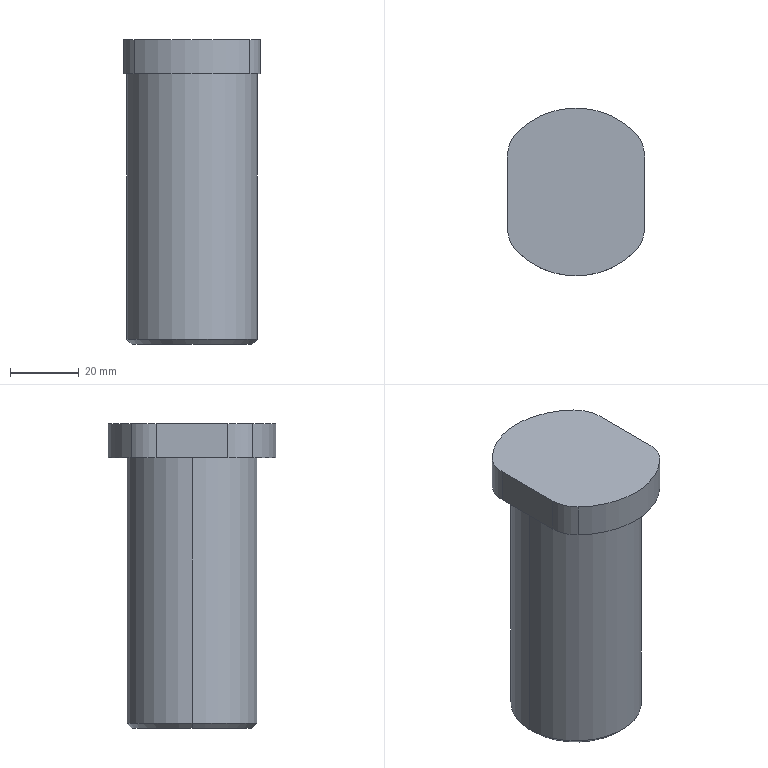Part | SolidWorks | features BaseBody 1 | 1 solid | 19 faces | box 40 x 49 x 89 mm | volume 90205 mm3 | cylinder 10 | plane 5 | cone 4 | commonest cylinder face diameters 20 x4 21 x2 38 x2 49 x2
STEP:
#1=CARTESIAN_POINT('',(-217.5,-135.,-429.5));
#2=VERTEX_POINT('',#1);
#3=CARTESIAN_POINT('',(-182.5,-135.,-429.5));
#4=VERTEX_POINT('',#3);
#5=CARTESIAN_POINT('',(-200.,-135.,-429.5));
#6=DIRECTION('',(0.,0.,-1.));
#7=DIRECTION('',(1.,0.,0.));
#8=AXIS2_PLACEMENT_3D('',#5,#6,#7);
#9=CIRCLE('',#8,17.5);
#10=EDGE_CURVE('',#2,#4,#9,.T.);
#11=ORIENTED_EDGE('',*,*,#10,.F.);
#12=CARTESIAN_POINT('',(-219.,-135.,-428.));
#13=VERTEX_POINT('',#12);
#14=CARTESIAN_POINT('',(-217.5,-135.,-429.5));
#15=DIRECTION('',(-0.7071,0.,0.7071));
#16=VECTOR('',#15,1000.);
#17=LINE('',#14,#16);
#18=EDGE_CURVE('',#2,#13,#17,.T.);
#19=ORIENTED_EDGE('',*,*,#18,.T.);
#20=CARTESIAN_POINT('',(-181.,-135.,-428.));
#21=VERTEX_POINT('',#20);
#22=CARTESIAN_POINT('',(-200.,-135.,-428.));
#23=DIRECTION('',(0.,0.,1.));
#24=DIRECTION('',(1.,0.,0.));
#25=AXIS2_PLACEMENT_3D('',#22,#23,#24);
#26=CIRCLE('',#25,19.);
#27=EDGE_CURVE('',#21,#13,#26,.T.);
#28=ORIENTED_EDGE('',*,*,#27,.F.);
#29=CARTESIAN_POINT('',(-182.5,-135.,-429.5));
#30=DIRECTION('',(0.7071,0.,0.7071));
#31=VECTOR('',#30,1000.);
#32=LINE('',#29,#31);
#33=EDGE_CURVE('',#4,#21,#32,.T.);
#34=ORIENTED_EDGE('',*,*,#33,.F.);
#35=EDGE_LOOP('',(#11,#19,#28,#34));
#36=FACE_OUTER_BOUND('',#35,.T.);
#37=CARTESIAN_POINT('',(-200.,-135.,-429.5));
#38=DIRECTION('',(0.,0.,1.));
#39=DIRECTION('',(1.,0.,0.));
#40=AXIS2_PLACEMENT_3D('',#37,#38,#39);
#41=CONICAL_SURFACE('',#40,17.5,0.7854);
#42=ADVANCED_FACE('',(#36),#41,.T.);
#43=CARTESIAN_POINT('',(-210.5,-135.,-429.5));
#44=VERTEX_POINT('',#43);
#45=CARTESIAN_POINT('',(-189.5,-135.,-429.5));
#46=VERTEX_POINT('',#45);
#47=CARTESIAN_POINT('',(-200.,-135.,-429.5));
#48=DIRECTION('',(0.,0.,1.));
#49=DIRECTION('',(1.,0.,0.));
#50=AXIS2_PLACEMENT_3D('',#47,#48,#49);
#51=CIRCLE('',#50,10.5);
#52=EDGE_CURVE('',#44,#46,#51,.T.);
#53=ORIENTED_EDGE('',*,*,#52,.F.);
#54=CARTESIAN_POINT('',(-210.5,-135.,-384.5));
#55=VERTEX_POINT('',#54);
#56=CARTESIAN_POINT('',(-210.5,-135.,-414.5));
#57=DIRECTION('',(0.,0.,1.));
#58=VECTOR('',#57,1000.);
#59=LINE('',#56,#58);
#60=EDGE_CURVE('',#44,#55,#59,.T.);
#61=ORIENTED_EDGE('',*,*,#60,.T.);
#62=CARTESIAN_POINT('',(-189.5,-135.,-384.5));
#63=VERTEX_POINT('',#62);
#64=CARTESIAN_POINT('',(-200.,-135.,-384.5));
#65=DIRECTION('',(0.,0.,1.));
#66=DIRECTION('',(1.,0.,0.));
#67=AXIS2_PLACEMENT_3D('',#64,#65,#66);
#68=CIRCLE('',#67,10.5);
#69=EDGE_CURVE('',#55,#63,#68,.T.);
#70=ORIENTED_EDGE('',*,*,#69,.T.);
#71=CARTESIAN_POINT('',(-189.5,-135.,-414.5));
#72=DIRECTION('',(0.,0.,1.));
#73=VECTOR('',#72,1000.);
#74=LINE('',#71,#73);
#75=EDGE_CURVE('',#46,#63,#74,.T.);
#76=ORIENTED_EDGE('',*,*,#75,.F.);
#77=EDGE_LOOP('',(#53,#61,#70,#76));
#78=FACE_OUTER_BOUND('',#77,.T.);
#79=CARTESIAN_POINT('',(-200.,-135.,-414.5));
#80=DIRECTION('',(0.,0.,1.));
#81=DIRECTION('',(1.,0.,0.));
#82=AXIS2_PLACEMENT_3D('',#79,#80,#81);
#83=CYLINDRICAL_SURFACE('',#82,10.5);
#84=ADVANCED_FACE('',(#78),#83,.F.);
#85=CARTESIAN_POINT('',(-200.,-135.,-378.191));
#86=VERTEX_POINT('',#85);
#87=CARTESIAN_POINT('',(-210.5,-135.,-384.5));
#88=DIRECTION('',(-0.8572,0.,-0.515));
#89=VECTOR('',#88,1000.);
#90=LINE('',#87,#89);
#91=EDGE_CURVE('',#86,#55,#90,.T.);
#92=ORIENTED_EDGE('',*,*,#91,.F.);
#93=CARTESIAN_POINT('',(-189.5,-135.,-384.5));
#94=DIRECTION('',(0.8572,0.,-0.515));
#95=VECTOR('',#94,1000.);
#96=LINE('',#93,#95);
#97=EDGE_CURVE('',#86,#63,#96,.T.);
#98=ORIENTED_EDGE('',*,*,#97,.T.);
#99=ORIENTED_EDGE('',*,*,#69,.F.);
#100=EDGE_LOOP('',(#92,#98,#99));
#101=FACE_OUTER_BOUND('',#100,.T.);
#102=CARTESIAN_POINT('',(-200.,-135.,-384.5));
#103=DIRECTION('',(0.,0.,-1.));
#104=DIRECTION('',(-1.,0.,0.));
#105=AXIS2_PLACEMENT_3D('',#102,#103,#104);
#106=CONICAL_SURFACE('',#105,10.5,1.03);
#107=ADVANCED_FACE('',(#101),#106,.F.);
#108=ORIENTED_EDGE('',*,*,#27,.T.);
#109=CARTESIAN_POINT('',(-219.,-135.,-350.5));
#110=VERTEX_POINT('',#109);
#111=CARTESIAN_POINT('',(-219.,-135.,-414.5));
#112=DIRECTION('',(0.,0.,1.));
#113=VECTOR('',#112,1000.);
#114=LINE('',#111,#113);
#115=EDGE_CURVE('',#13,#110,#114,.T.);
#116=ORIENTED_EDGE('',*,*,#115,.T.);
#117=CARTESIAN_POINT('',(-181.,-135.,-350.5));
#118=VERTEX_POINT('',#117);
#119=CARTESIAN_POINT('',(-200.,-135.,-350.5));
#120=DIRECTION('',(0.,0.,-1.));
#121=DIRECTION('',(1.,0.,0.));
#122=AXIS2_PLACEMENT_3D('',#119,#120,#121);
#123=CIRCLE('',#122,19.);
#124=EDGE_CURVE('',#110,#118,#123,.T.);
#125=ORIENTED_EDGE('',*,*,#124,.T.);
#126=CARTESIAN_POINT('',(-181.,-135.,-414.5));
#127=DIRECTION('',(0.,0.,1.));
#128=VECTOR('',#127,1000.);
#129=LINE('',#126,#128);
#130=EDGE_CURVE('',#21,#118,#129,.T.);
#131=ORIENTED_EDGE('',*,*,#130,.F.);
#132=EDGE_LOOP('',(#108,#116,#125,#131));
#133=FACE_OUTER_BOUND('',#132,.T.);
#134=CARTESIAN_POINT('',(-200.,-135.,-414.5));
#135=DIRECTION('',(0.,0.,1.));
#136=DIRECTION('',(1.,0.,0.));
#137=AXIS2_PLACEMENT_3D('',#134,#135,#136);
#138=CYLINDRICAL_SURFACE('',#137,19.);
#139=ADVANCED_FACE('',(#133),#138,.T.);
#140=ORIENTED_EDGE('',*,*,#115,.F.);
#141=CARTESIAN_POINT('',(-200.,-135.,-428.));
#142=DIRECTION('',(0.,0.,1.));
#143=DIRECTION('',(1.,0.,0.));
#144=AXIS2_PLACEMENT_3D('',#141,#142,#143);
#145=CIRCLE('',#144,19.);
#146=EDGE_CURVE('',#13,#21,#145,.T.);
#147=ORIENTED_EDGE('',*,*,#146,.T.);
#148=ORIENTED_EDGE('',*,*,#130,.T.);
#149=CARTESIAN_POINT('',(-200.,-135.,-350.5));
#150=DIRECTION('',(0.,0.,-1.));
#151=DIRECTION('',(1.,0.,0.));
#152=AXIS2_PLACEMENT_3D('',#149,#150,#151);
#153=CIRCLE('',#152,19.);
#154=EDGE_CURVE('',#118,#110,#153,.T.);
#155=ORIENTED_EDGE('',*,*,#154,.T.);
#156=EDGE_LOOP('',(#140,#147,#148,#155));
#157=FACE_OUTER_BOUND('',#156,.T.);
#158=CARTESIAN_POINT('',(-200.,-135.,-414.5));
#159=DIRECTION('',(0.,0.,1.));
#160=DIRECTION('',(1.,0.,0.));
#161=AXIS2_PLACEMENT_3D('',#158,#159,#160);
#162=CYLINDRICAL_SURFACE('',#161,19.);
#163=ADVANCED_FACE('',(#157),#162,.T.);
#164=CARTESIAN_POINT('',(-200.,-135.,-429.5));
#165=DIRECTION('',(0.,0.,-1.));
#166=DIRECTION('',(1.,0.,0.));
#167=AXIS2_PLACEMENT_3D('',#164,#165,#166);
#168=CIRCLE('',#167,17.5);
#169=EDGE_CURVE('',#4,#2,#168,.T.);
#170=ORIENTED_EDGE('',*,*,#169,.T.);
#171=ORIENTED_EDGE('',*,*,#10,.T.);
#172=EDGE_LOOP('',(#170,#171));
#173=FACE_OUTER_BOUND('',#172,.T.);
#174=CARTESIAN_POINT('',(-200.,-135.,-429.5));
#175=DIRECTION('',(0.,0.,1.));
#176=DIRECTION('',(1.,0.,0.));
#177=AXIS2_PLACEMENT_3D('',#174,#175,#176);
#178=CIRCLE('',#177,10.5);
#179=EDGE_CURVE('',#46,#44,#178,.T.);
#180=ORIENTED_EDGE('',*,*,#179,.T.);
#181=ORIENTED_EDGE('',*,*,#52,.T.);
#182=EDGE_LOOP('',(#180,#181));
#183=FACE_BOUND('',#182,.T.);
#184=CARTESIAN_POINT('',(-200.,-135.,-429.5));
#185=DIRECTION('',(0.,0.,1.));
#186=DIRECTION('',(1.,0.,0.));
#187=AXIS2_PLACEMENT_3D('',#184,#185,#186);
#188=PLANE('',#187);
#189=ADVANCED_FACE('',(#173,#183),#188,.F.);
#190=CARTESIAN_POINT('',(-220.,-124.5,-350.5));
#191=VERTEX_POINT('',#190);
#192=CARTESIAN_POINT('',(-220.,-145.5,-350.5));
#193=VERTEX_POINT('',#192);
#194=CARTESIAN_POINT('',(-220.,-118.387,-350.5));
#195=DIRECTION('',(0.,-1.,0.));
#196=VECTOR('',#195,1000.);
#197=LINE('',#194,#196);
#198=EDGE_CURVE('',#191,#193,#197,.T.);
#199=ORIENTED_EDGE('',*,*,#198,.T.);
#200=CARTESIAN_POINT('',(-220.,-145.5,-340.5));
#201=VERTEX_POINT('',#200);
#202=CARTESIAN_POINT('',(-220.,-145.5,-350.5));
#203=DIRECTION('',(0.,0.,1.));
#204=VECTOR('',#203,1000.);
#205=LINE('',#202,#204);
#206=EDGE_CURVE('',#193,#201,#205,.T.);
#207=ORIENTED_EDGE('',*,*,#206,.T.);
#208=CARTESIAN_POINT('',(-220.,-124.5,-340.5));
#209=VERTEX_POINT('',#208);
#210=CARTESIAN_POINT('',(-220.,-118.387,-340.5));
#211=DIRECTION('',(0.,-1.,0.));
#212=VECTOR('',#211,1000.);
#213=LINE('',#210,#212);
#214=EDGE_CURVE('',#209,#201,#213,.T.);
#215=ORIENTED_EDGE('',*,*,#214,.F.);
#216=CARTESIAN_POINT('',(-220.,-124.5,-350.5));
#217=DIRECTION('',(0.,0.,-1.));
#218=VECTOR('',#217,1000.);
#219=LINE('',#216,#218);
#220=EDGE_CURVE('',#209,#191,#219,.T.);
#221=ORIENTED_EDGE('',*,*,#220,.T.);
#222=EDGE_LOOP('',(#199,#207,#215,#221));
#223=FACE_OUTER_BOUND('',#222,.T.);
#224=CARTESIAN_POINT('',(-220.,-118.387,-350.5));
#225=DIRECTION('',(-1.,0.,0.));
#226=DIRECTION('',(0.,-1.,0.));
#227=AXIS2_PLACEMENT_3D('',#224,#225,#226);
#228=PLANE('',#227);
#229=ADVANCED_FACE('',(#223),#228,.T.);
#230=CARTESIAN_POINT('',(-216.897,-152.741,-350.5));
#231=VERTEX_POINT('',#230);
#232=CARTESIAN_POINT('',(-183.103,-152.741,-350.5));
#233=VERTEX_POINT('',#232);
#234=CARTESIAN_POINT('',(-200.,-135.,-350.5));
#235=DIRECTION('',(0.,0.,1.));
#236=DIRECTION('',(1.,0.,0.));
#237=AXIS2_PLACEMENT_3D('',#234,#235,#236);
#238=CIRCLE('',#237,24.5);
#239=EDGE_CURVE('',#231,#233,#238,.T.);
#240=ORIENTED_EDGE('',*,*,#239,.T.);
#241=CARTESIAN_POINT('',(-183.103,-152.741,-340.5));
#242=VERTEX_POINT('',#241);
#243=CARTESIAN_POINT('',(-183.103,-152.741,-350.5));
#244=DIRECTION('',(0.,0.,1.));
#245=VECTOR('',#244,1000.);
#246=LINE('',#243,#245);
#247=EDGE_CURVE('',#233,#242,#246,.T.);
#248=ORIENTED_EDGE('',*,*,#247,.T.);
#249=CARTESIAN_POINT('',(-216.897,-152.741,-340.5));
#250=VERTEX_POINT('',#249);
#251=CARTESIAN_POINT('',(-200.,-135.,-340.5));
#252=DIRECTION('',(0.,0.,1.));
#253=DIRECTION('',(1.,0.,0.));
#254=AXIS2_PLACEMENT_3D('',#251,#252,#253);
#255=CIRCLE('',#254,24.5);
#256=EDGE_CURVE('',#250,#242,#255,.T.);
#257=ORIENTED_EDGE('',*,*,#256,.F.);
#258=CARTESIAN_POINT('',(-216.897,-152.741,-350.5));
#259=DIRECTION('',(0.,0.,-1.));
#260=VECTOR('',#259,1000.);
#261=LINE('',#258,#260);
#262=EDGE_CURVE('',#250,#231,#261,.T.);
#263=ORIENTED_EDGE('',*,*,#262,.T.);
#264=EDGE_LOOP('',(#240,#248,#257,#263));
#265=FACE_OUTER_BOUND('',#264,.T.);
#266=CARTESIAN_POINT('',(-200.,-135.,-350.5));
#267=DIRECTION('',(0.,0.,1.));
#268=DIRECTION('',(1.,0.,0.));
#269=AXIS2_PLACEMENT_3D('',#266,#267,#268);
#270=CYLINDRICAL_SURFACE('',#269,24.5);
#271=ADVANCED_FACE('',(#265),#270,.T.);
#272=CARTESIAN_POINT('',(-180.,-145.5,-350.5));
#273=VERTEX_POINT('',#272);
#274=CARTESIAN_POINT('',(-180.,-124.5,-350.5));
#275=VERTEX_POINT('',#274);
#276=CARTESIAN_POINT('',(-180.,-151.613,-350.5));
#277=DIRECTION('',(0.,1.,0.));
#278=VECTOR('',#277,1000.);
#279=LINE('',#276,#278);
#280=EDGE_CURVE('',#273,#275,#279,.T.);
#281=ORIENTED_EDGE('',*,*,#280,.T.);
#282=CARTESIAN_POINT('',(-180.,-124.5,-340.5));
#283=VERTEX_POINT('',#282);
#284=CARTESIAN_POINT('',(-180.,-124.5,-350.5));
#285=DIRECTION('',(0.,0.,1.));
#286=VECTOR('',#285,1000.);
#287=LINE('',#284,#286);
#288=EDGE_CURVE('',#275,#283,#287,.T.);
#289=ORIENTED_EDGE('',*,*,#288,.T.);
#290=CARTESIAN_POINT('',(-180.,-145.5,-340.5));
#291=VERTEX_POINT('',#290);
#292=CARTESIAN_POINT('',(-180.,-151.613,-340.5));
#293=DIRECTION('',(0.,1.,0.));
#294=VECTOR('',#293,1000.);
#295=LINE('',#292,#294);
#296=EDGE_CURVE('',#291,#283,#295,.T.);
#297=ORIENTED_EDGE('',*,*,#296,.F.);
#298=CARTESIAN_POINT('',(-180.,-145.5,-350.5));
#299=DIRECTION('',(0.,0.,-1.));
#300=VECTOR('',#299,1000.);
#301=LINE('',#298,#300);
#302=EDGE_CURVE('',#291,#273,#301,.T.);
#303=ORIENTED_EDGE('',*,*,#302,.T.);
#304=EDGE_LOOP('',(#281,#289,#297,#303));
#305=FACE_OUTER_BOUND('',#304,.T.);
#306=CARTESIAN_POINT('',(-180.,-151.613,-350.5));
#307=DIRECTION('',(1.,0.,0.));
#308=DIRECTION('',(0.,1.,0.));
#309=AXIS2_PLACEMENT_3D('',#306,#307,#308);
#310=PLANE('',#309);
#311=ADVANCED_FACE('',(#305),#310,.T.);
#312=CARTESIAN_POINT('',(-183.103,-117.259,-340.5));
#313=VERTEX_POINT('',#312);
#314=CARTESIAN_POINT('',(-216.897,-117.259,-340.5));
#315=VERTEX_POINT('',#314);
#316=CARTESIAN_POINT('',(-200.,-135.,-340.5));
#317=DIRECTION('',(0.,0.,1.));
#318=DIRECTION('',(1.,0.,0.));
#319=AXIS2_PLACEMENT_3D('',#316,#317,#318);
#320=CIRCLE('',#319,24.5);
#321=EDGE_CURVE('',#313,#315,#320,.T.);
#322=ORIENTED_EDGE('',*,*,#321,.F.);
#323=CARTESIAN_POINT('',(-183.103,-117.259,-350.5));
#324=VERTEX_POINT('',#323);
#325=CARTESIAN_POINT('',(-183.103,-117.259,-350.5));
#326=DIRECTION('',(0.,0.,-1.));
#327=VECTOR('',#326,1000.);
#328=LINE('',#325,#327);
#329=EDGE_CURVE('',#313,#324,#328,.T.);
#330=ORIENTED_EDGE('',*,*,#329,.T.);
#331=CARTESIAN_POINT('',(-216.897,-117.259,-350.5));
#332=VERTEX_POINT('',#331);
#333=CARTESIAN_POINT('',(-200.,-135.,-350.5));
#334=DIRECTION('',(0.,0.,1.));
#335=DIRECTION('',(1.,0.,0.));
#336=AXIS2_PLACEMENT_3D('',#333,#334,#335);
#337=CIRCLE('',#336,24.5);
#338=EDGE_CURVE('',#324,#332,#337,.T.);
#339=ORIENTED_EDGE('',*,*,#338,.T.);
#340=CARTESIAN_POINT('',(-216.897,-117.259,-350.5));
#341=DIRECTION('',(0.,0.,1.));
#342=VECTOR('',#341,1000.);
#343=LINE('',#340,#342);
#344=EDGE_CURVE('',#332,#315,#343,.T.);
#345=ORIENTED_EDGE('',*,*,#344,.T.);
#346=EDGE_LOOP('',(#322,#330,#339,#345));
#347=FACE_OUTER_BOUND('',#346,.T.);
#348=CARTESIAN_POINT('',(-200.,-135.,-350.5));
#349=DIRECTION('',(0.,0.,1.));
#350=DIRECTION('',(1.,0.,0.));
#351=AXIS2_PLACEMENT_3D('',#348,#349,#350);
#352=CYLINDRICAL_SURFACE('',#351,24.5);
#353=ADVANCED_FACE('',(#347),#352,.T.);
#354=ORIENTED_EDGE('',*,*,#154,.F.);
#355=ORIENTED_EDGE('',*,*,#124,.F.);
#356=EDGE_LOOP('',(#354,#355));
#357=FACE_BOUND('',#356,.T.);
#358=ORIENTED_EDGE('',*,*,#338,.F.);
#359=CARTESIAN_POINT('',(-190.,-124.5,-350.5));
#360=DIRECTION('',(0.,0.,-1.));
#361=DIRECTION('',(1.,0.,0.));
#362=AXIS2_PLACEMENT_3D('',#359,#360,#361);
#363=CIRCLE('',#362,10.);
#364=EDGE_CURVE('',#324,#275,#363,.T.);
#365=ORIENTED_EDGE('',*,*,#364,.T.);
#366=ORIENTED_EDGE('',*,*,#280,.F.);
#367=CARTESIAN_POINT('',(-190.,-145.5,-350.5));
#368=DIRECTION('',(0.,0.,-1.));
#369=DIRECTION('',(1.,0.,0.));
#370=AXIS2_PLACEMENT_3D('',#367,#368,#369);
#371=CIRCLE('',#370,10.);
#372=EDGE_CURVE('',#273,#233,#371,.T.);
#373=ORIENTED_EDGE('',*,*,#372,.T.);
#374=ORIENTED_EDGE('',*,*,#239,.F.);
#375=CARTESIAN_POINT('',(-210.,-145.5,-350.5));
#376=DIRECTION('',(0.,0.,-1.));
#377=DIRECTION('',(1.,0.,0.));
#378=AXIS2_PLACEMENT_3D('',#375,#376,#377);
#379=CIRCLE('',#378,10.);
#380=EDGE_CURVE('',#231,#193,#379,.T.);
#381=ORIENTED_EDGE('',*,*,#380,.T.);
#382=ORIENTED_EDGE('',*,*,#198,.F.);
#383=CARTESIAN_POINT('',(-210.,-124.5,-350.5));
#384=DIRECTION('',(0.,0.,-1.));
#385=DIRECTION('',(1.,0.,0.));
#386=AXIS2_PLACEMENT_3D('',#383,#384,#385);
#387=CIRCLE('',#386,10.);
#388=EDGE_CURVE('',#191,#332,#387,.T.);
#389=ORIENTED_EDGE('',*,*,#388,.T.);
#390=EDGE_LOOP('',(#358,#365,#366,#373,#374,#381,#382,#389));
#391=FACE_OUTER_BOUND('',#390,.T.);
#392=CARTESIAN_POINT('',(-200.,-135.,-350.5));
#393=DIRECTION('',(0.,0.,1.));
#394=DIRECTION('',(1.,0.,0.));
#395=AXIS2_PLACEMENT_3D('',#392,#393,#394);
#396=PLANE('',#395);
#397=ADVANCED_FACE('',(#357,#391),#396,.F.);
#398=ORIENTED_EDGE('',*,*,#296,.T.);
#399=CARTESIAN_POINT('',(-190.,-124.5,-340.5));
#400=DIRECTION('',(0.,0.,1.));
#401=DIRECTION('',(1.,0.,0.));
#402=AXIS2_PLACEMENT_3D('',#399,#400,#401);
#403=CIRCLE('',#402,10.);
#404=EDGE_CURVE('',#283,#313,#403,.T.);
#405=ORIENTED_EDGE('',*,*,#404,.T.);
#406=ORIENTED_EDGE('',*,*,#321,.T.);
#407=CARTESIAN_POINT('',(-210.,-124.5,-340.5));
#408=DIRECTION('',(0.,0.,1.));
#409=DIRECTION('',(1.,0.,0.));
#410=AXIS2_PLACEMENT_3D('',#407,#408,#409);
#411=CIRCLE('',#410,10.);
#412=EDGE_CURVE('',#315,#209,#411,.T.);
#413=ORIENTED_EDGE('',*,*,#412,.T.);
#414=ORIENTED_EDGE('',*,*,#214,.T.);
#415=CARTESIAN_POINT('',(-210.,-145.5,-340.5));
#416=DIRECTION('',(0.,0.,1.));
#417=DIRECTION('',(1.,0.,0.));
#418=AXIS2_PLACEMENT_3D('',#415,#416,#417);
#419=CIRCLE('',#418,10.);
#420=EDGE_CURVE('',#201,#250,#419,.T.);
#421=ORIENTED_EDGE('',*,*,#420,.T.);
#422=ORIENTED_EDGE('',*,*,#256,.T.);
#423=CARTESIAN_POINT('',(-190.,-145.5,-340.5));
#424=DIRECTION('',(0.,0.,1.));
#425=DIRECTION('',(1.,0.,0.));
#426=AXIS2_PLACEMENT_3D('',#423,#424,#425);
#427=CIRCLE('',#426,10.);
#428=EDGE_CURVE('',#242,#291,#427,.T.);
#429=ORIENTED_EDGE('',*,*,#428,.T.);
#430=EDGE_LOOP('',(#398,#405,#406,#413,#414,#421,#422,#429));
#431=FACE_OUTER_BOUND('',#430,.T.);
#432=CARTESIAN_POINT('',(-200.,-135.,-340.5));
#433=DIRECTION('',(0.,0.,1.));
#434=DIRECTION('',(1.,0.,0.));
#435=AXIS2_PLACEMENT_3D('',#432,#433,#434);
#436=PLANE('',#435);
#437=ADVANCED_FACE('',(#431),#436,.T.);
#438=ORIENTED_EDGE('',*,*,#97,.F.);
#439=ORIENTED_EDGE('',*,*,#91,.T.);
#440=CARTESIAN_POINT('',(-200.,-135.,-384.5));
#441=DIRECTION('',(0.,0.,1.));
#442=DIRECTION('',(1.,0.,0.));
#443=AXIS2_PLACEMENT_3D('',#440,#441,#442);
#444=CIRCLE('',#443,10.5);
#445=EDGE_CURVE('',#63,#55,#444,.T.);
#446=ORIENTED_EDGE('',*,*,#445,.F.);
#447=EDGE_LOOP('',(#438,#439,#446));
#448=FACE_OUTER_BOUND('',#447,.T.);
#449=CARTESIAN_POINT('',(-200.,-135.,-384.5));
#450=DIRECTION('',(0.,0.,-1.));
#451=DIRECTION('',(-1.,0.,0.));
#452=AXIS2_PLACEMENT_3D('',#449,#450,#451);
#453=CONICAL_SURFACE('',#452,10.5,1.03);
#454=ADVANCED_FACE('',(#448),#453,.F.);
#455=ORIENTED_EDGE('',*,*,#60,.F.);
#456=ORIENTED_EDGE('',*,*,#179,.F.);
#457=ORIENTED_EDGE('',*,*,#75,.T.);
#458=ORIENTED_EDGE('',*,*,#445,.T.);
#459=EDGE_LOOP('',(#455,#456,#457,#458));
#460=FACE_OUTER_BOUND('',#459,.T.);
#461=CARTESIAN_POINT('',(-200.,-135.,-414.5));
#462=DIRECTION('',(0.,0.,1.));
#463=DIRECTION('',(1.,0.,0.));
#464=AXIS2_PLACEMENT_3D('',#461,#462,#463);
#465=CYLINDRICAL_SURFACE('',#464,10.5);
#466=ADVANCED_FACE('',(#460),#465,.F.);
#467=ORIENTED_EDGE('',*,*,#18,.F.);
#468=ORIENTED_EDGE('',*,*,#169,.F.);
#469=ORIENTED_EDGE('',*,*,#33,.T.);
#470=ORIENTED_EDGE('',*,*,#146,.F.);
#471=EDGE_LOOP('',(#467,#468,#469,#470));
#472=FACE_OUTER_BOUND('',#471,.T.);
#473=CARTESIAN_POINT('',(-200.,-135.,-429.5));
#474=DIRECTION('',(0.,0.,1.));
#475=DIRECTION('',(1.,0.,0.));
#476=AXIS2_PLACEMENT_3D('',#473,#474,#475);
#477=CONICAL_SURFACE('',#476,17.5,0.7854);
#478=ADVANCED_FACE('',(#472),#477,.T.);
#479=ORIENTED_EDGE('',*,*,#364,.F.);
#480=ORIENTED_EDGE('',*,*,#329,.F.);
#481=ORIENTED_EDGE('',*,*,#404,.F.);
#482=ORIENTED_EDGE('',*,*,#288,.F.);
#483=EDGE_LOOP('',(#479,#480,#481,#482));
#484=FACE_OUTER_BOUND('',#483,.T.);
#485=CARTESIAN_POINT('',(-190.,-124.5,-350.5));
#486=DIRECTION('',(0.,0.,1.));
#487=DIRECTION('',(1.,0.,0.));
#488=AXIS2_PLACEMENT_3D('',#485,#486,#487);
#489=CYLINDRICAL_SURFACE('',#488,10.);
#490=ADVANCED_FACE('',(#484),#489,.T.);
#491=ORIENTED_EDGE('',*,*,#372,.F.);
#492=ORIENTED_EDGE('',*,*,#302,.F.);
#493=ORIENTED_EDGE('',*,*,#428,.F.);
#494=ORIENTED_EDGE('',*,*,#247,.F.);
#495=EDGE_LOOP('',(#491,#492,#493,#494));
#496=FACE_OUTER_BOUND('',#495,.T.);
#497=CARTESIAN_POINT('',(-190.,-145.5,-350.5));
#498=DIRECTION('',(0.,0.,1.));
#499=DIRECTION('',(1.,0.,0.));
#500=AXIS2_PLACEMENT_3D('',#497,#498,#499);
#501=CYLINDRICAL_SURFACE('',#500,10.);
#502=ADVANCED_FACE('',(#496),#501,.T.);
#503=ORIENTED_EDGE('',*,*,#380,.F.);
#504=ORIENTED_EDGE('',*,*,#262,.F.);
#505=ORIENTED_EDGE('',*,*,#420,.F.);
#506=ORIENTED_EDGE('',*,*,#206,.F.);
#507=EDGE_LOOP('',(#503,#504,#505,#506));
#508=FACE_OUTER_BOUND('',#507,.T.);
#509=CARTESIAN_POINT('',(-210.,-145.5,-350.5));
#510=DIRECTION('',(0.,0.,1.));
#511=DIRECTION('',(1.,0.,0.));
#512=AXIS2_PLACEMENT_3D('',#509,#510,#511);
#513=CYLINDRICAL_SURFACE('',#512,10.);
#514=ADVANCED_FACE('',(#508),#513,.T.);
#515=ORIENTED_EDGE('',*,*,#388,.F.);
#516=ORIENTED_EDGE('',*,*,#220,.F.);
#517=ORIENTED_EDGE('',*,*,#412,.F.);
#518=ORIENTED_EDGE('',*,*,#344,.F.);
#519=EDGE_LOOP('',(#515,#516,#517,#518));
#520=FACE_OUTER_BOUND('',#519,.T.);
#521=CARTESIAN_POINT('',(-210.,-124.5,-350.5));
#522=DIRECTION('',(0.,0.,1.));
#523=DIRECTION('',(1.,0.,0.));
#524=AXIS2_PLACEMENT_3D('',#521,#522,#523);
#525=CYLINDRICAL_SURFACE('',#524,10.);
#526=ADVANCED_FACE('',(#520),#525,.T.);
#527=CLOSED_SHELL('',(#42,#84,#107,#139,#163,#189,#229,#271,#311,#353,#397,#437,#454,#466,#478,#490,#502,#514,#526));
#528=MANIFOLD_SOLID_BREP('',#527);
#529=CARTESIAN_POINT('',(0.,0.,0.));
#530=DIRECTION('',(0.,0.,1.));
#531=DIRECTION('',(1.,0.,0.));
#532=AXIS2_PLACEMENT_3D('',#529,#530,#531);
#533=(LENGTH_UNIT()NAMED_UNIT(*)SI_UNIT(.MILLI.,.METRE.));
#534=UNCERTAINTY_MEASURE_WITH_UNIT(LENGTH_MEASURE(0.00001),#533,'','');
#535=(NAMED_UNIT(*)PLANE_ANGLE_UNIT()SI_UNIT($,.RADIAN.));
#536=(NAMED_UNIT(*)SI_UNIT($,.STERADIAN.)SOLID_ANGLE_UNIT());
#537=(GEOMETRIC_REPRESENTATION_CONTEXT(3)GLOBAL_UNCERTAINTY_ASSIGNED_CONTEXT((#534))GLOBAL_UNIT_ASSIGNED_CONTEXT((#533,#535,#536))REPRESENTATION_CONTEXT('',''));
#538=ADVANCED_BREP_SHAPE_REPRESENTATION('',(#528,#532),#537);